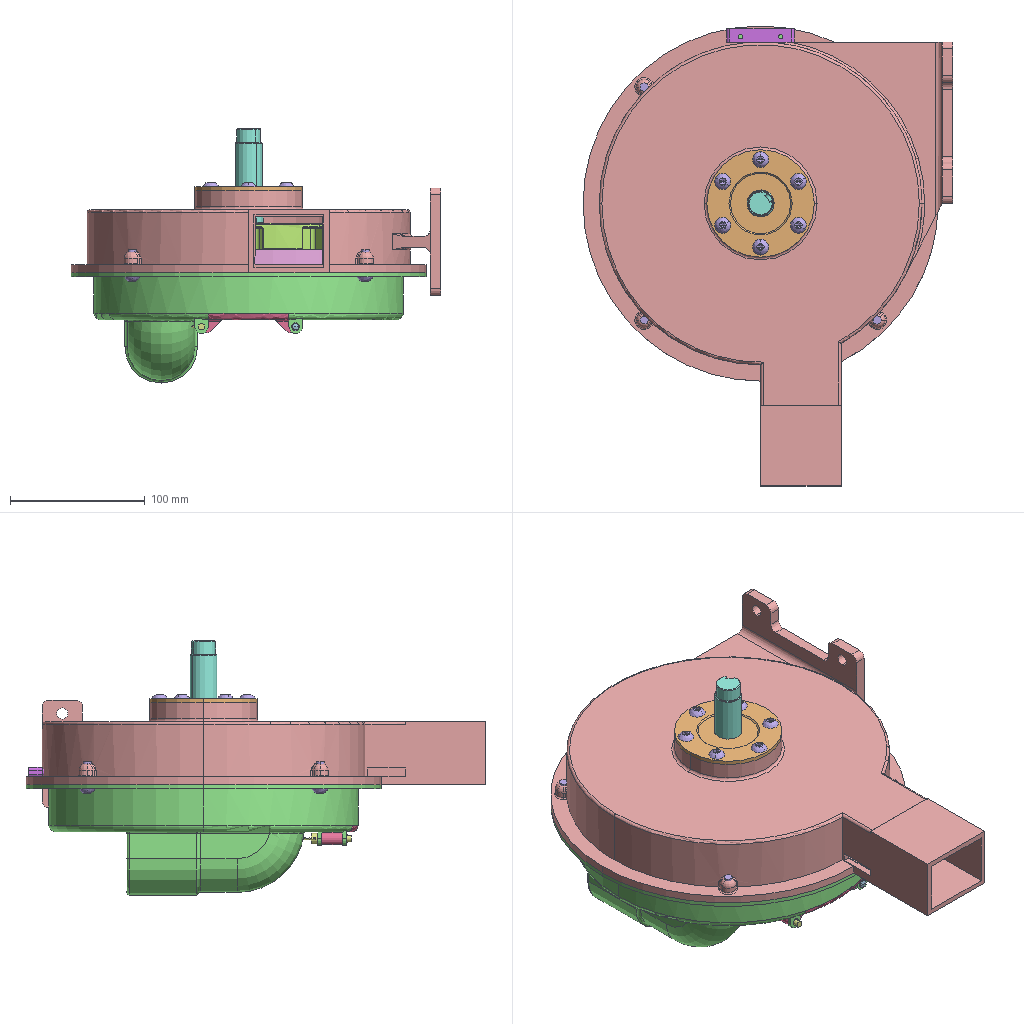Assembly | SolidWorks | 20 different items | 51 placed | box 275 x 342 x 189 mm
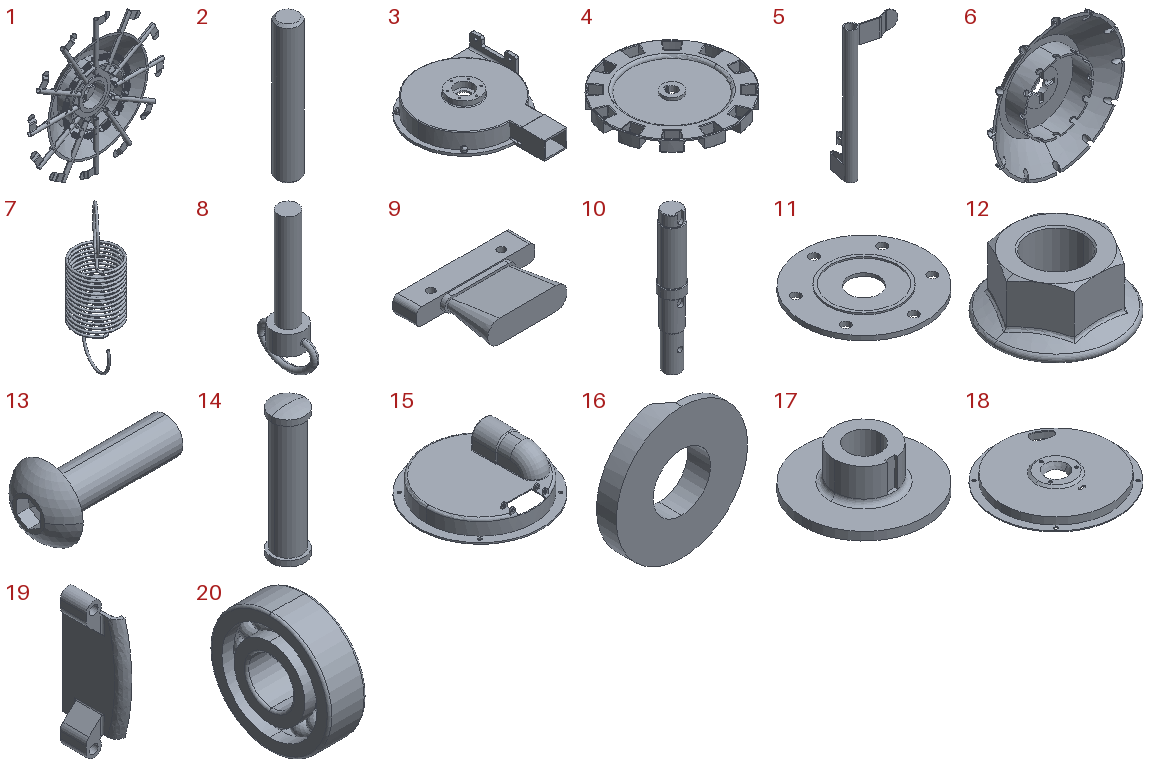Parts list (item | name | quantity | parent item | size | volume | features):
1 | (subassembly) | x1 | - | 212 x 28.613 x 212 mm | 113831 mm3 | features ReferencePattern 22, LocalCirPattern 2
2 | - | x1 | - | 5 x 5 x 30 mm | 585.383 mm3 | features Chamfer 1, Extrusion 1
3 | - | x1 | - | 275 x 342 x 80 mm | 622085 mm3 | features ICE 11, Fillet 10, BossThin 3, CirPattern 3, 3DProfileFeature 2, Cut 2, HoleWzd 2, Revolution 1
4 | - | x1 | - | 220 x 220 x 20 mm | 250365 mm3 | features Fillet 5, ICE 5, CirPattern 2, Revolution 1
5 | - | x12 | in 1 | 26.854 x 14.962 x 75 mm | 843.538 mm3 | features BossThin 3, 3DProfileFeature 1, Extrusion 1, Fillet 1, HoleWzd 1, ICE 1
6 | - | x1 | in 1 | 160 x 27 x 160 mm | 59816 mm3 | features ICE 6, CirPattern 3, Revolution 1, Shell 1
7 | - | x12 | in 1 | 6.3 x 6.3 x 20.605 mm | 22.571 mm3 | features 3DProfileFeature 2, MacroFeature 1
8 | - | x1 | - | 8 x 15.16 x 35.75 mm | 789.697 mm3 | features Extrusion 1, ICE 1, Sweep 1
9 | - | x1 | - | 50 x 32 x 9.622 mm | 7730 mm3 | features ICE 2, 3DProfileFeature 1, Extrusion 1, Fillet 1, HoleWzd 1
10 | - | x1 | - | 22 x 22 x 135 mm | 36047 mm3 | features ICE 9, Chamfer 2, Extrusion 1
11 | - | x1 | - | 80 x 80 x 4 mm | 12563 mm3 | features ICE 4, Chamfer 1, CirPattern 1, Extrusion 1
12 | - | x1 | - | 42.8 x 42.8 x 20 mm | 12206 mm3 | features RevCut 3, Extrusion 1, Fillet 1, LPattern 1, Revolution 1
13 | - | x10 | - | 23.3 x 12 x 12 mm | 775.96 mm3 | features Cut 2, RevCut 2, Boss 1, Extrusion 1, Fillet 1, LPattern 1
14 | - | x1 | - | 6 x 6 x 24 mm | 483.151 mm3 | features Dome 2, ICE 2, Extrusion 1
15 | - | x1 | - | 264 x 264 x 82 mm | 198550 mm3 | features Fillet 6, ICE 6, Sweep 2, CirPattern 1, CombineBodies 1, Cut 1, Extrusion 1, MirrorPattern 1, Shell 1
16 | - | x1 | in 1 | 80 x 14 x 80 mm | 43623 mm3 | features ICE 3, Chamfer 1, Extrusion 1, Helix 1, SweepCut 1
17 | - | x1 | - | 74 x 74 x 25 mm | 32918 mm3 | features ICE 3, Extrusion 1, Fillet 1
18 | - | x1 | - | 260 x 260 x 21 mm | 125361 mm3 | features ICE 5, CirPattern 2, 3DProfileFeature 1, HoleWzd 1, Revolution 1
19 | - | x1 | - | 14.5 x 35.129 x 79 mm | 7419 mm3 | features ICE 4, Fillet 2, Sweep 2, MirrorPattern 1
20 | - | x1 | - | 8 x 26 x 26 mm | 2684 mm3 | features Revolution 3, CirPattern 1, Fillet 1
Mates (type | each side: item.copy, entity, surface, feature):
In the top assembly
Concentric | 3.1 face cylinder Cut-Extrude1 | 20.1 face cylinder Revolve3
Coincident | 3.1 face plane Cut-Extrude1 | 20.1 face plane Revolve3
Concentric | 3.1 face cylinder Cut-Extrude2 | 4.1 face cylinder Cut-Extrude1
DistanceDim | 4.1 face plane Revolve1 | 3.1 face plane Revolve1
Coincident | 3.1 face plane Revolve1 | 18.1 face plane Revolve1
Concentric | 20.1 face cylinder Revolve2 | 10.1 face cylinder Boss-Extrude3
Coincident | 4.1 face plane Revolve1 | 10.1 face plane Boss-Extrude1
Coincident | 4.1 face plane Cut-Extrude3 | 10.1 face plane Cut-Extrude2
Concentric | 3.1 face cylinder Revolve1 | 11.1 face cylinder Boss-Extrude1
Coincident | 3.1 face plane Revolve1 | 11.1 face plane Boss-Extrude1
Concentric | 3.1 face cylinder M5 Tapped Hole1 | 11.1 face cylinder Cut-Extrude2
Concentric | 11.1 face cylinder Cut-Extrude2 | 13.1 face cylinder BaseBody
Coincident | 11.1 face plane Boss-Extrude1 | 13.1 face plane BaseHead
Concentric | 3.1 face cylinder Revolve1 | 15.1 face cylinder Boss-Extrude1
Concentric | 15.1 face cylinder Cut-Extrude6 | 19.1 face cylinder Boss-Extrude1
Coincident | 15.1 face plane Boss-Extrude4 | 19.1 face plane Boss-Extrude1
LimitPlanarAngleDim | 19.1 face plane Sweep1 | 15.1 face plane Boss-Extrude1
Concentric | 15.1 face cylinder Cut-Extrude6 | 14.1 face cylinder Boss-Extrude2
Coincident | 15.1 face plane Boss-Extrude4 | 14.1 face plane Boss-Extrude2
Concentric | 15.1 face cylinder Mirror1 | 8.1 face cylinder Boss-Extrude2
LimitDistanceDim | 8.1 face plane Boss-Extrude1 | 15.1 face plane Mirror1
Parallel | 15.1 face plane Boss-Extrude1 | 8.1 plane
Concentric | 3.1 face cylinder Revolve1 | 18.1 face cylinder Revolve1
Coincident | 18.1 plane | assembly plane
Coincident | 3.1 face plane Cut-Extrude9 | 9.1 face plane Boss-Extrude2
Tangent | 3.1 face cylinder Revolve1 | 9.1 face plane Boss-Extrude1
Concentric | 18.1 edge | 17.1 face cylinder Boss-Extrude2
Coincident | 18.1 face plane Revolve1 | 17.1 face plane Boss-Extrude1
Coincident | 10.1 plane | 1.1 plane
Concentric | 10.1 face cylinder Boss-Extrude7 | 16.1 face cylinder Boss-Extrude2
Coincident | 18.1 face plane Revolve1 | 6.1 face plane Revolve1
Coincident | 17.1 face plane Cut-Extrude2 | 16.1 face plane Boss-Extrude3
Concentric | 10.1 face cylinder Cut-Extrude3 | 2.1 face cylinder Boss-Extrude1
DistanceDim | 2.1 face plane Boss-Extrude1 | 6.1 face plane Cut-Extrude3
Coincident | 17.1 plane | assembly plane
Concentric | 6.1 face cylinder Cut-Extrude2 | 12.1 face cone Hole
Coincident | 6.1 face plane Boss-Extrude3 | 12.1 face plane BaseNut
Coincident | 15.1 plane | assembly plane
Coincident | 3.1 face plane Revolve1 | 15.1 face plane Boss-Extrude1
Concentric | 15.1 face cylinder Cut-Extrude7 | 13.2 face cylinder BaseBody
Coincident | 15.1 face plane Boss-Extrude5 | 13.2 face plane BaseHead
In subassembly 1
Concentric | 6.2 face cylinder Cut-Extrude2 | 16.2 face cylinder Boss-Extrude2
Coincident | 6.2 face plane Boss-Extrude3 | 16.2 face plane Boss-Extrude1
Concentric | 6.2 face cylinder Cut-Extrude1 | 5.1 face cylinder Boss-Extrude1
DistanceDim | 5.1 face plane Boss-Extrude1 | 1.2 plane
Lock | 5.2 select_type:0 | 7.1 select_type:0